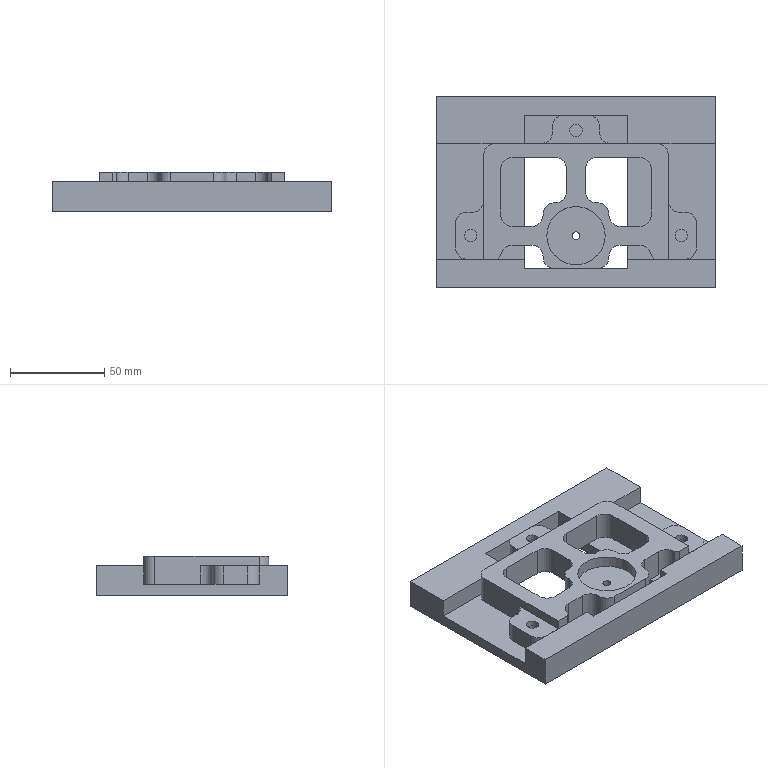NC program | NX | posted with a generic post | part box 148 x 101.5 x 21 mm
Lines 1 to 23 of 5700:
N10 G17 G21 G94 G90
(FLOOR_WALL , TOOL : D63)
N12 T01 M6
N14 G54
N16 G17 G0 G90 X101.5 Y-42.747 S6500 M3
N18 G43 Z30. H1
N20 Z4.
N22 G94 G1 Z1. F1500.
N24 X98.5
N26 X-98.5
N28 Y-34.204
N30 Y-12.599
N32 X98.5
N34 Y17.55
N36 X-98.5
N38 X-101.5
N40 Z4.
N42 G0 Z30.
N44 M5